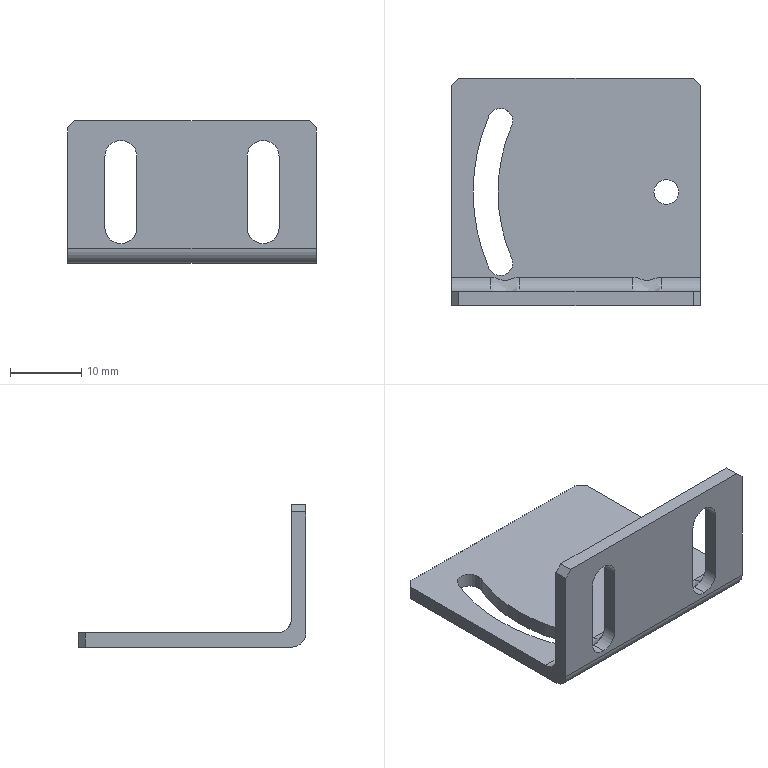Part | STEP file | 1 solid | 36 faces | box 35 x 32 x 20 mm | volume 3068 mm3 | cylinder 18 | plane 16 | spline 2 | commonest cylinder face diameters 4.5 x6 3.5 x4 4 x4 47.3 x2 54.3 x2